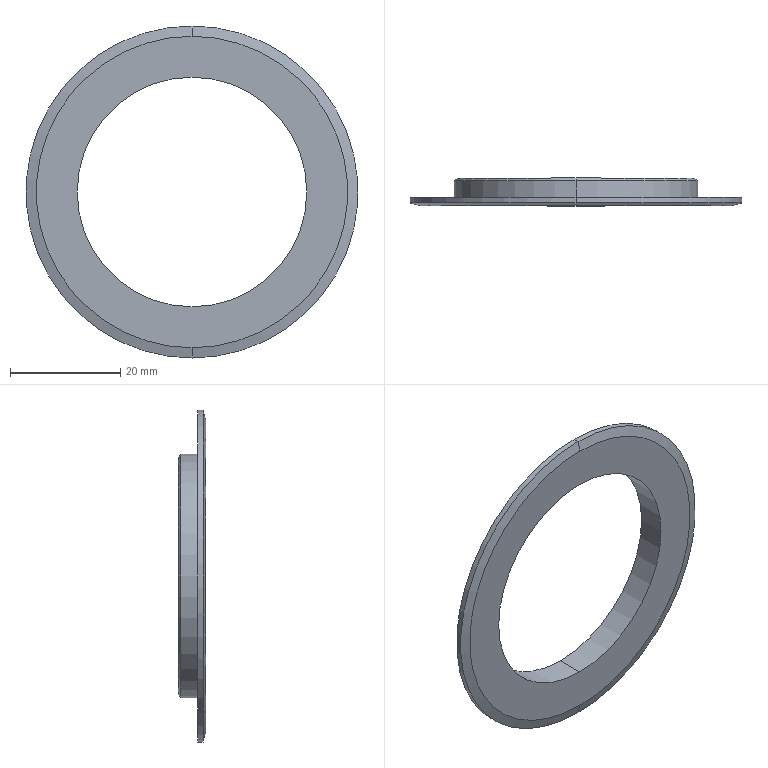Part | SolidWorks | features Chamfer 2, Extrusion 1, ICE 1 | 1 solid | 13 faces | box 60.296 x 5 x 60.296 mm | volume 2721 mm3 | cylinder 6 | cone 4 | plane 3 | commonest cylinder face diameters 41.7 x2 44.2 x2 60.296 x2
STEP:
#1=CARTESIAN_POINT('',(0.,0.,-28.282));
#2=VERTEX_POINT('',#1);
#3=CARTESIAN_POINT('',(0.,0.,28.282));
#4=VERTEX_POINT('',#3);
#5=CARTESIAN_POINT('',(0.,0.,0.));
#6=DIRECTION('',(0.,-1.,0.));
#7=DIRECTION('',(0.,0.,1.));
#8=AXIS2_PLACEMENT_3D('',#5,#6,#7);
#9=CIRCLE('',#8,28.282);
#10=EDGE_CURVE('',#2,#4,#9,.T.);
#11=ORIENTED_EDGE('',*,*,#10,.F.);
#12=CARTESIAN_POINT('',(0.,0.5,-30.148));
#13=VERTEX_POINT('',#12);
#14=CARTESIAN_POINT('',(0.,0.5,-30.148));
#15=DIRECTION('',(0.,0.2588,-0.9659));
#16=VECTOR('',#15,1000.);
#17=LINE('',#14,#16);
#18=EDGE_CURVE('',#2,#13,#17,.T.);
#19=ORIENTED_EDGE('',*,*,#18,.T.);
#20=CARTESIAN_POINT('',(0.,0.5,30.148));
#21=VERTEX_POINT('',#20);
#22=CARTESIAN_POINT('',(0.,0.5,0.));
#23=DIRECTION('',(0.,1.,0.));
#24=DIRECTION('',(0.,0.,1.));
#25=AXIS2_PLACEMENT_3D('',#22,#23,#24);
#26=CIRCLE('',#25,30.148);
#27=EDGE_CURVE('',#21,#13,#26,.T.);
#28=ORIENTED_EDGE('',*,*,#27,.F.);
#29=CARTESIAN_POINT('',(0.,0.5,30.148));
#30=DIRECTION('',(0.,0.2588,0.9659));
#31=VECTOR('',#30,1000.);
#32=LINE('',#29,#31);
#33=EDGE_CURVE('',#4,#21,#32,.T.);
#34=ORIENTED_EDGE('',*,*,#33,.F.);
#35=EDGE_LOOP('',(#11,#19,#28,#34));
#36=FACE_OUTER_BOUND('',#35,.T.);
#37=CARTESIAN_POINT('',(0.,0.5,0.));
#38=DIRECTION('',(0.,1.,0.));
#39=DIRECTION('',(0.,0.,1.));
#40=AXIS2_PLACEMENT_3D('',#37,#38,#39);
#41=CONICAL_SURFACE('',#40,30.148,1.309);
#42=ADVANCED_FACE('',(#36),#41,.T.);
#43=CARTESIAN_POINT('',(0.,5.,21.6));
#44=VERTEX_POINT('',#43);
#45=CARTESIAN_POINT('',(0.,5.,-21.6));
#46=VERTEX_POINT('',#45);
#47=CARTESIAN_POINT('',(0.,5.,0.));
#48=DIRECTION('',(0.,1.,0.));
#49=DIRECTION('',(0.,0.,1.));
#50=AXIS2_PLACEMENT_3D('',#47,#48,#49);
#51=CIRCLE('',#50,21.6);
#52=EDGE_CURVE('',#44,#46,#51,.T.);
#53=ORIENTED_EDGE('',*,*,#52,.F.);
#54=CARTESIAN_POINT('',(0.,4.5,22.1));
#55=VERTEX_POINT('',#54);
#56=CARTESIAN_POINT('',(0.,5.,21.6));
#57=DIRECTION('',(0.,-0.7071,0.7071));
#58=VECTOR('',#57,1000.);
#59=LINE('',#56,#58);
#60=EDGE_CURVE('',#44,#55,#59,.T.);
#61=ORIENTED_EDGE('',*,*,#60,.T.);
#62=CARTESIAN_POINT('',(0.,4.5,-22.1));
#63=VERTEX_POINT('',#62);
#64=CARTESIAN_POINT('',(0.,4.5,0.));
#65=DIRECTION('',(0.,-1.,0.));
#66=DIRECTION('',(0.,0.,1.));
#67=AXIS2_PLACEMENT_3D('',#64,#65,#66);
#68=CIRCLE('',#67,22.1);
#69=EDGE_CURVE('',#63,#55,#68,.T.);
#70=ORIENTED_EDGE('',*,*,#69,.F.);
#71=CARTESIAN_POINT('',(0.,5.,-21.6));
#72=DIRECTION('',(0.,-0.7071,-0.7071));
#73=VECTOR('',#72,1000.);
#74=LINE('',#71,#73);
#75=EDGE_CURVE('',#46,#63,#74,.T.);
#76=ORIENTED_EDGE('',*,*,#75,.F.);
#77=EDGE_LOOP('',(#53,#61,#70,#76));
#78=FACE_OUTER_BOUND('',#77,.T.);
#79=CARTESIAN_POINT('',(0.,5.,0.));
#80=DIRECTION('',(0.,-1.,0.));
#81=DIRECTION('',(0.,0.,-1.));
#82=AXIS2_PLACEMENT_3D('',#79,#80,#81);
#83=CONICAL_SURFACE('',#82,21.6,0.7854);
#84=ADVANCED_FACE('',(#78),#83,.T.);
#85=ORIENTED_EDGE('',*,*,#69,.T.);
#86=CARTESIAN_POINT('',(0.,1.5,22.1));
#87=VERTEX_POINT('',#86);
#88=CARTESIAN_POINT('',(0.,5.,22.1));
#89=DIRECTION('',(0.,-1.,0.));
#90=VECTOR('',#89,1000.);
#91=LINE('',#88,#90);
#92=EDGE_CURVE('',#55,#87,#91,.T.);
#93=ORIENTED_EDGE('',*,*,#92,.T.);
#94=CARTESIAN_POINT('',(0.,1.5,-22.1));
#95=VERTEX_POINT('',#94);
#96=CARTESIAN_POINT('',(0.,1.5,0.));
#97=DIRECTION('',(0.,1.,0.));
#98=DIRECTION('',(0.,0.,1.));
#99=AXIS2_PLACEMENT_3D('',#96,#97,#98);
#100=CIRCLE('',#99,22.1);
#101=EDGE_CURVE('',#87,#95,#100,.T.);
#102=ORIENTED_EDGE('',*,*,#101,.T.);
#103=CARTESIAN_POINT('',(0.,5.,-22.1));
#104=DIRECTION('',(0.,-1.,0.));
#105=VECTOR('',#104,1000.);
#106=LINE('',#103,#105);
#107=EDGE_CURVE('',#63,#95,#106,.T.);
#108=ORIENTED_EDGE('',*,*,#107,.F.);
#109=EDGE_LOOP('',(#85,#93,#102,#108));
#110=FACE_OUTER_BOUND('',#109,.T.);
#111=CARTESIAN_POINT('',(0.,5.,0.));
#112=DIRECTION('',(0.,-1.,0.));
#113=DIRECTION('',(0.,0.,-1.));
#114=AXIS2_PLACEMENT_3D('',#111,#112,#113);
#115=CYLINDRICAL_SURFACE('',#114,22.1);
#116=ADVANCED_FACE('',(#110),#115,.T.);
#117=CARTESIAN_POINT('',(0.,5.,-20.85));
#118=VERTEX_POINT('',#117);
#119=CARTESIAN_POINT('',(0.,5.,20.85));
#120=VERTEX_POINT('',#119);
#121=CARTESIAN_POINT('',(0.,5.,0.));
#122=DIRECTION('',(0.,1.,0.));
#123=DIRECTION('',(0.,0.,1.));
#124=AXIS2_PLACEMENT_3D('',#121,#122,#123);
#125=CIRCLE('',#124,20.85);
#126=EDGE_CURVE('',#118,#120,#125,.T.);
#127=ORIENTED_EDGE('',*,*,#126,.T.);
#128=CARTESIAN_POINT('',(0.,0.,20.85));
#129=VERTEX_POINT('',#128);
#130=CARTESIAN_POINT('',(0.,1.5,20.85));
#131=DIRECTION('',(0.,-1.,0.));
#132=VECTOR('',#131,1000.);
#133=LINE('',#130,#132);
#134=EDGE_CURVE('',#120,#129,#133,.T.);
#135=ORIENTED_EDGE('',*,*,#134,.T.);
#136=CARTESIAN_POINT('',(0.,0.,-20.85));
#137=VERTEX_POINT('',#136);
#138=CARTESIAN_POINT('',(0.,0.,0.));
#139=DIRECTION('',(0.,1.,0.));
#140=DIRECTION('',(0.,0.,1.));
#141=AXIS2_PLACEMENT_3D('',#138,#139,#140);
#142=CIRCLE('',#141,20.85);
#143=EDGE_CURVE('',#137,#129,#142,.T.);
#144=ORIENTED_EDGE('',*,*,#143,.F.);
#145=CARTESIAN_POINT('',(0.,1.5,-20.85));
#146=DIRECTION('',(0.,-1.,0.));
#147=VECTOR('',#146,1000.);
#148=LINE('',#145,#147);
#149=EDGE_CURVE('',#118,#137,#148,.T.);
#150=ORIENTED_EDGE('',*,*,#149,.F.);
#151=EDGE_LOOP('',(#127,#135,#144,#150));
#152=FACE_OUTER_BOUND('',#151,.T.);
#153=CARTESIAN_POINT('',(0.,1.5,0.));
#154=DIRECTION('',(0.,-1.,0.));
#155=DIRECTION('',(0.,0.,-1.));
#156=AXIS2_PLACEMENT_3D('',#153,#154,#155);
#157=CYLINDRICAL_SURFACE('',#156,20.85);
#158=ADVANCED_FACE('',(#152),#157,.F.);
#159=CARTESIAN_POINT('',(0.,1.5,30.148));
#160=VERTEX_POINT('',#159);
#161=CARTESIAN_POINT('',(0.,1.5,-30.148));
#162=VERTEX_POINT('',#161);
#163=CARTESIAN_POINT('',(0.,1.5,0.));
#164=DIRECTION('',(0.,1.,0.));
#165=DIRECTION('',(0.,0.,1.));
#166=AXIS2_PLACEMENT_3D('',#163,#164,#165);
#167=CIRCLE('',#166,30.148);
#168=EDGE_CURVE('',#160,#162,#167,.T.);
#169=ORIENTED_EDGE('',*,*,#168,.F.);
#170=CARTESIAN_POINT('',(0.,1.5,30.148));
#171=DIRECTION('',(0.,-1.,0.));
#172=VECTOR('',#171,1000.);
#173=LINE('',#170,#172);
#174=EDGE_CURVE('',#160,#21,#173,.T.);
#175=ORIENTED_EDGE('',*,*,#174,.T.);
#176=ORIENTED_EDGE('',*,*,#27,.T.);
#177=CARTESIAN_POINT('',(0.,1.5,-30.148));
#178=DIRECTION('',(0.,-1.,0.));
#179=VECTOR('',#178,1000.);
#180=LINE('',#177,#179);
#181=EDGE_CURVE('',#162,#13,#180,.T.);
#182=ORIENTED_EDGE('',*,*,#181,.F.);
#183=EDGE_LOOP('',(#169,#175,#176,#182));
#184=FACE_OUTER_BOUND('',#183,.T.);
#185=CARTESIAN_POINT('',(0.,1.5,0.));
#186=DIRECTION('',(0.,-1.,0.));
#187=DIRECTION('',(0.,0.,-1.));
#188=AXIS2_PLACEMENT_3D('',#185,#186,#187);
#189=CYLINDRICAL_SURFACE('',#188,30.148);
#190=ADVANCED_FACE('',(#184),#189,.T.);
#191=CARTESIAN_POINT('',(0.,1.5,0.));
#192=DIRECTION('',(0.,1.,0.));
#193=DIRECTION('',(0.,0.,1.));
#194=AXIS2_PLACEMENT_3D('',#191,#192,#193);
#195=CIRCLE('',#194,30.148);
#196=EDGE_CURVE('',#162,#160,#195,.T.);
#197=ORIENTED_EDGE('',*,*,#196,.T.);
#198=ORIENTED_EDGE('',*,*,#168,.T.);
#199=EDGE_LOOP('',(#197,#198));
#200=FACE_OUTER_BOUND('',#199,.T.);
#201=CARTESIAN_POINT('',(0.,1.5,0.));
#202=DIRECTION('',(0.,1.,0.));
#203=DIRECTION('',(0.,0.,1.));
#204=AXIS2_PLACEMENT_3D('',#201,#202,#203);
#205=CIRCLE('',#204,22.1);
#206=EDGE_CURVE('',#95,#87,#205,.T.);
#207=ORIENTED_EDGE('',*,*,#206,.F.);
#208=ORIENTED_EDGE('',*,*,#101,.F.);
#209=EDGE_LOOP('',(#207,#208));
#210=FACE_BOUND('',#209,.T.);
#211=CARTESIAN_POINT('',(0.,1.5,0.));
#212=DIRECTION('',(0.,1.,0.));
#213=DIRECTION('',(0.,0.,1.));
#214=AXIS2_PLACEMENT_3D('',#211,#212,#213);
#215=PLANE('',#214);
#216=ADVANCED_FACE('',(#200,#210),#215,.T.);
#217=CARTESIAN_POINT('',(0.,0.,0.));
#218=DIRECTION('',(0.,-1.,0.));
#219=DIRECTION('',(0.,0.,1.));
#220=AXIS2_PLACEMENT_3D('',#217,#218,#219);
#221=CIRCLE('',#220,28.282);
#222=EDGE_CURVE('',#4,#2,#221,.T.);
#223=ORIENTED_EDGE('',*,*,#222,.T.);
#224=ORIENTED_EDGE('',*,*,#10,.T.);
#225=EDGE_LOOP('',(#223,#224));
#226=FACE_OUTER_BOUND('',#225,.T.);
#227=ORIENTED_EDGE('',*,*,#143,.T.);
#228=CARTESIAN_POINT('',(0.,0.,0.));
#229=DIRECTION('',(0.,1.,0.));
#230=DIRECTION('',(0.,0.,1.));
#231=AXIS2_PLACEMENT_3D('',#228,#229,#230);
#232=CIRCLE('',#231,20.85);
#233=EDGE_CURVE('',#129,#137,#232,.T.);
#234=ORIENTED_EDGE('',*,*,#233,.T.);
#235=EDGE_LOOP('',(#227,#234));
#236=FACE_BOUND('',#235,.T.);
#237=CARTESIAN_POINT('',(0.,0.,0.));
#238=DIRECTION('',(0.,1.,0.));
#239=DIRECTION('',(0.,0.,1.));
#240=AXIS2_PLACEMENT_3D('',#237,#238,#239);
#241=PLANE('',#240);
#242=ADVANCED_FACE('',(#226,#236),#241,.F.);
#243=ORIENTED_EDGE('',*,*,#174,.F.);
#244=ORIENTED_EDGE('',*,*,#196,.F.);
#245=ORIENTED_EDGE('',*,*,#181,.T.);
#246=CARTESIAN_POINT('',(0.,0.5,0.));
#247=DIRECTION('',(0.,1.,0.));
#248=DIRECTION('',(0.,0.,1.));
#249=AXIS2_PLACEMENT_3D('',#246,#247,#248);
#250=CIRCLE('',#249,30.148);
#251=EDGE_CURVE('',#13,#21,#250,.T.);
#252=ORIENTED_EDGE('',*,*,#251,.T.);
#253=EDGE_LOOP('',(#243,#244,#245,#252));
#254=FACE_OUTER_BOUND('',#253,.T.);
#255=CARTESIAN_POINT('',(0.,1.5,0.));
#256=DIRECTION('',(0.,-1.,0.));
#257=DIRECTION('',(0.,0.,-1.));
#258=AXIS2_PLACEMENT_3D('',#255,#256,#257);
#259=CYLINDRICAL_SURFACE('',#258,30.148);
#260=ADVANCED_FACE('',(#254),#259,.T.);
#261=ORIENTED_EDGE('',*,*,#134,.F.);
#262=CARTESIAN_POINT('',(0.,5.,0.));
#263=DIRECTION('',(0.,1.,0.));
#264=DIRECTION('',(0.,0.,1.));
#265=AXIS2_PLACEMENT_3D('',#262,#263,#264);
#266=CIRCLE('',#265,20.85);
#267=EDGE_CURVE('',#120,#118,#266,.T.);
#268=ORIENTED_EDGE('',*,*,#267,.T.);
#269=ORIENTED_EDGE('',*,*,#149,.T.);
#270=ORIENTED_EDGE('',*,*,#233,.F.);
#271=EDGE_LOOP('',(#261,#268,#269,#270));
#272=FACE_OUTER_BOUND('',#271,.T.);
#273=CARTESIAN_POINT('',(0.,1.5,0.));
#274=DIRECTION('',(0.,-1.,0.));
#275=DIRECTION('',(0.,0.,-1.));
#276=AXIS2_PLACEMENT_3D('',#273,#274,#275);
#277=CYLINDRICAL_SURFACE('',#276,20.85);
#278=ADVANCED_FACE('',(#272),#277,.F.);
#279=CARTESIAN_POINT('',(0.,5.,0.));
#280=DIRECTION('',(0.,1.,0.));
#281=DIRECTION('',(0.,0.,1.));
#282=AXIS2_PLACEMENT_3D('',#279,#280,#281);
#283=CIRCLE('',#282,21.6);
#284=EDGE_CURVE('',#46,#44,#283,.T.);
#285=ORIENTED_EDGE('',*,*,#284,.T.);
#286=ORIENTED_EDGE('',*,*,#52,.T.);
#287=EDGE_LOOP('',(#285,#286));
#288=FACE_OUTER_BOUND('',#287,.T.);
#289=ORIENTED_EDGE('',*,*,#126,.F.);
#290=ORIENTED_EDGE('',*,*,#267,.F.);
#291=EDGE_LOOP('',(#289,#290));
#292=FACE_BOUND('',#291,.T.);
#293=CARTESIAN_POINT('',(0.,5.,0.));
#294=DIRECTION('',(0.,1.,0.));
#295=DIRECTION('',(0.,0.,1.));
#296=AXIS2_PLACEMENT_3D('',#293,#294,#295);
#297=PLANE('',#296);
#298=ADVANCED_FACE('',(#288,#292),#297,.T.);
#299=ORIENTED_EDGE('',*,*,#92,.F.);
#300=CARTESIAN_POINT('',(0.,4.5,0.));
#301=DIRECTION('',(0.,-1.,0.));
#302=DIRECTION('',(0.,0.,1.));
#303=AXIS2_PLACEMENT_3D('',#300,#301,#302);
#304=CIRCLE('',#303,22.1);
#305=EDGE_CURVE('',#55,#63,#304,.T.);
#306=ORIENTED_EDGE('',*,*,#305,.T.);
#307=ORIENTED_EDGE('',*,*,#107,.T.);
#308=ORIENTED_EDGE('',*,*,#206,.T.);
#309=EDGE_LOOP('',(#299,#306,#307,#308));
#310=FACE_OUTER_BOUND('',#309,.T.);
#311=CARTESIAN_POINT('',(0.,5.,0.));
#312=DIRECTION('',(0.,-1.,0.));
#313=DIRECTION('',(0.,0.,-1.));
#314=AXIS2_PLACEMENT_3D('',#311,#312,#313);
#315=CYLINDRICAL_SURFACE('',#314,22.1);
#316=ADVANCED_FACE('',(#310),#315,.T.);
#317=ORIENTED_EDGE('',*,*,#60,.F.);
#318=ORIENTED_EDGE('',*,*,#284,.F.);
#319=ORIENTED_EDGE('',*,*,#75,.T.);
#320=ORIENTED_EDGE('',*,*,#305,.F.);
#321=EDGE_LOOP('',(#317,#318,#319,#320));
#322=FACE_OUTER_BOUND('',#321,.T.);
#323=CARTESIAN_POINT('',(0.,5.,0.));
#324=DIRECTION('',(0.,-1.,0.));
#325=DIRECTION('',(0.,0.,-1.));
#326=AXIS2_PLACEMENT_3D('',#323,#324,#325);
#327=CONICAL_SURFACE('',#326,21.6,0.7854);
#328=ADVANCED_FACE('',(#322),#327,.T.);
#329=ORIENTED_EDGE('',*,*,#18,.F.);
#330=ORIENTED_EDGE('',*,*,#222,.F.);
#331=ORIENTED_EDGE('',*,*,#33,.T.);
#332=ORIENTED_EDGE('',*,*,#251,.F.);
#333=EDGE_LOOP('',(#329,#330,#331,#332));
#334=FACE_OUTER_BOUND('',#333,.T.);
#335=CARTESIAN_POINT('',(0.,0.5,0.));
#336=DIRECTION('',(0.,1.,0.));
#337=DIRECTION('',(0.,0.,1.));
#338=AXIS2_PLACEMENT_3D('',#335,#336,#337);
#339=CONICAL_SURFACE('',#338,30.148,1.309);
#340=ADVANCED_FACE('',(#334),#339,.T.);
#341=CLOSED_SHELL('',(#42,#84,#116,#158,#190,#216,#242,#260,#278,#298,#316,#328,#340));
#342=MANIFOLD_SOLID_BREP('',#341);
#343=CARTESIAN_POINT('',(0.,0.,0.));
#344=DIRECTION('',(0.,0.,1.));
#345=DIRECTION('',(1.,0.,0.));
#346=AXIS2_PLACEMENT_3D('',#343,#344,#345);
#347=(LENGTH_UNIT()NAMED_UNIT(*)SI_UNIT(.MILLI.,.METRE.));
#348=UNCERTAINTY_MEASURE_WITH_UNIT(LENGTH_MEASURE(0.00001),#347,'','');
#349=(NAMED_UNIT(*)PLANE_ANGLE_UNIT()SI_UNIT($,.RADIAN.));
#350=(NAMED_UNIT(*)SI_UNIT($,.STERADIAN.)SOLID_ANGLE_UNIT());
#351=(GEOMETRIC_REPRESENTATION_CONTEXT(3)GLOBAL_UNCERTAINTY_ASSIGNED_CONTEXT((#348))GLOBAL_UNIT_ASSIGNED_CONTEXT((#347,#349,#350))REPRESENTATION_CONTEXT('',''));
#352=ADVANCED_BREP_SHAPE_REPRESENTATION('',(#342,#346),#351);